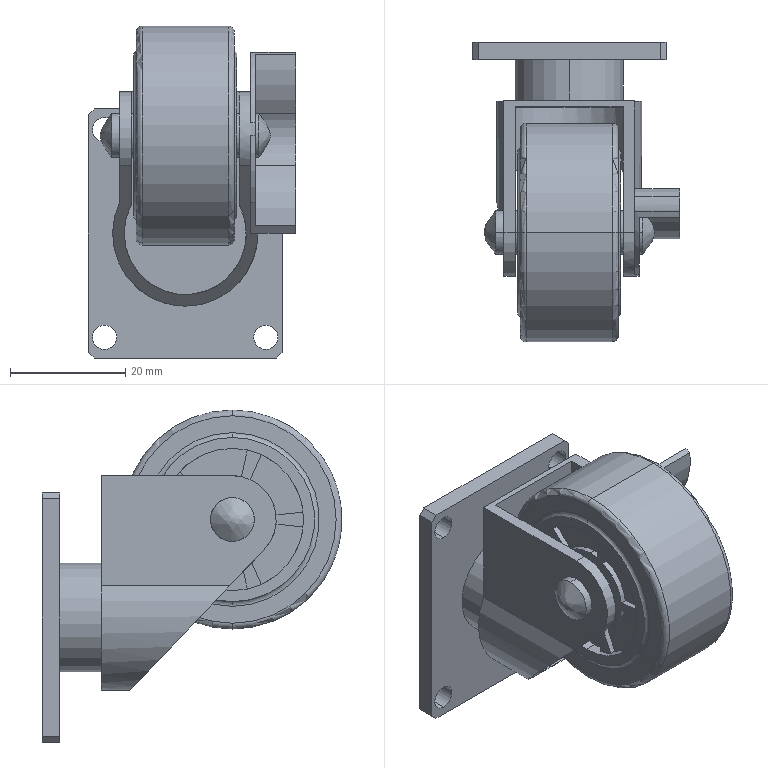Part | NX | features BREP 1, DATUM_CSYS 1 | 1 solid | 123 faces | box 35.944 x 52 x 57.6 mm | volume 28894 mm3 | plane 61 | cylinder 48 | torus 12 | spline 2 | commonest cylinder face diameters 15.2 x15 4.2 x8 7.6 x8 24.7 x4 18.9 x2 33.44 x2